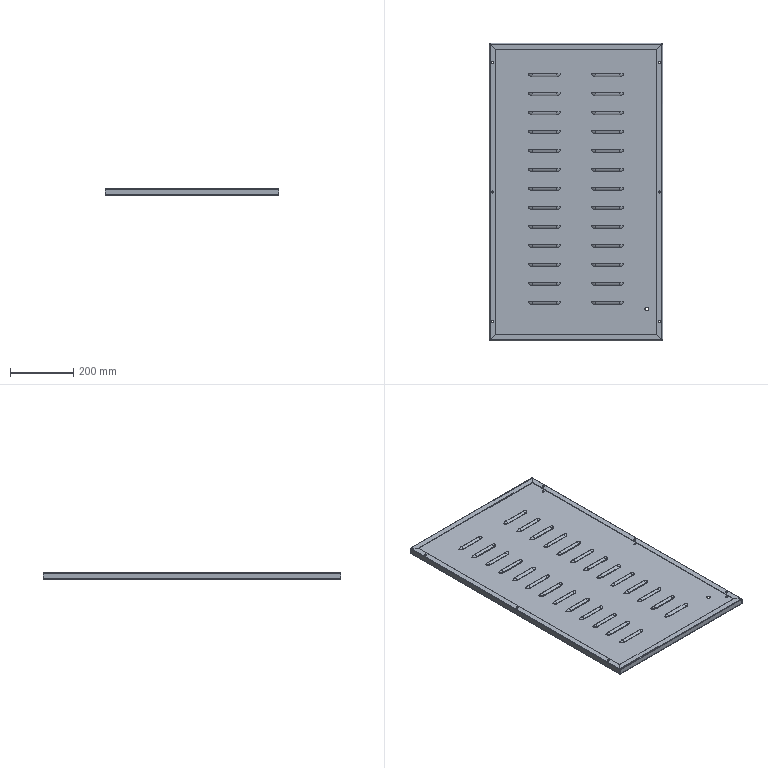Part | SolidWorks | features EdgeFlange 2, FlatPattern 1, FormToolInstance 1, ICE 1, SMBaseFlange 1, SheetMetal 1 | 1 solid | 564 faces | box 548 x 940 x 20 mm | volume 744289 mm3 | torus 208 | cylinder 146 | spline 120 | plane 90 | commonest cylinder face diameters 3.6 x26 6 x26 29 x26 31.4 x26 6.5 x24 2 x8